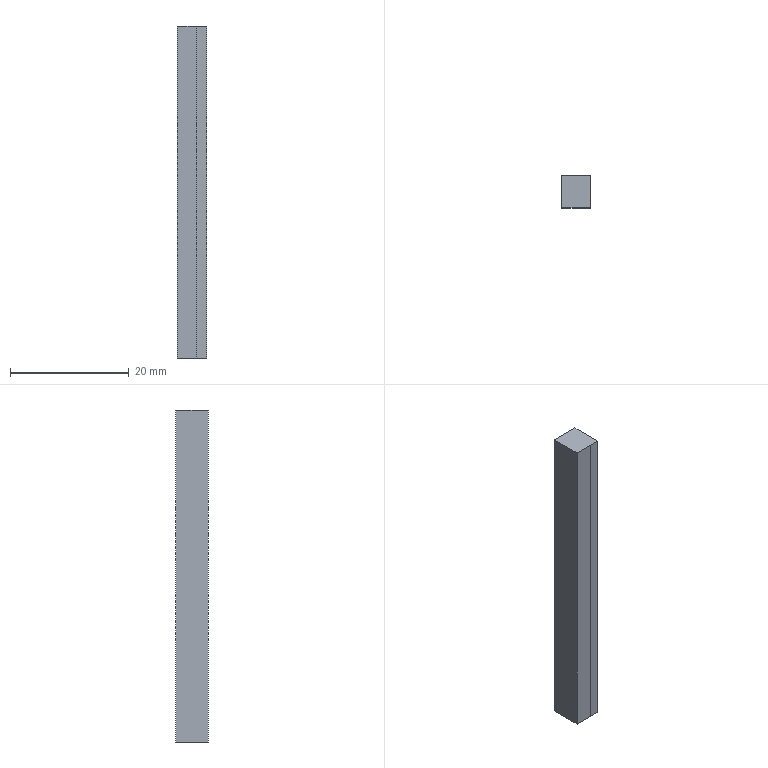Part | NX | features BREP 2 | 2 solids | 14 faces | box 4.903 x 5.406 x 56 mm | volume 2968 mm3 | plane 14
STEP:
#1=CARTESIAN_POINT('',(2.452,2.703,-4.));
#2=VERTEX_POINT('',#1);
#3=CARTESIAN_POINT('',(2.452,2.703,52.));
#4=VERTEX_POINT('',#3);
#5=CARTESIAN_POINT('',(2.452,2.703,0.));
#6=DIRECTION('',(0.,0.,1.));
#7=VECTOR('',#6,1000.);
#8=LINE('',#5,#7);
#9=EDGE_CURVE('',#2,#4,#8,.T.);
#10=ORIENTED_EDGE('',*,*,#9,.T.);
#11=CARTESIAN_POINT('',(2.452,-2.697,52.));
#12=VERTEX_POINT('',#11);
#13=CARTESIAN_POINT('',(2.452,24.305,52.));
#14=DIRECTION('',(0.,1.,0.));
#15=VECTOR('',#14,1000.);
#16=LINE('',#13,#15);
#17=EDGE_CURVE('',#12,#4,#16,.T.);
#18=ORIENTED_EDGE('',*,*,#17,.F.);
#19=CARTESIAN_POINT('',(2.452,-2.697,-4.));
#20=VERTEX_POINT('',#19);
#21=CARTESIAN_POINT('',(2.452,-2.697,0.));
#22=DIRECTION('',(0.,0.,1.));
#23=VECTOR('',#22,1000.);
#24=LINE('',#21,#23);
#25=EDGE_CURVE('',#20,#12,#24,.T.);
#26=ORIENTED_EDGE('',*,*,#25,.F.);
#27=CARTESIAN_POINT('',(2.452,24.305,-4.));
#28=DIRECTION('',(0.,1.,0.));
#29=VECTOR('',#28,1000.);
#30=LINE('',#27,#29);
#31=EDGE_CURVE('',#20,#2,#30,.T.);
#32=ORIENTED_EDGE('',*,*,#31,.T.);
#33=EDGE_LOOP('',(#10,#18,#26,#32));
#34=FACE_BOUND('',#33,.T.);
#35=CARTESIAN_POINT('',(2.452,2.703,0.));
#36=DIRECTION('',(-1.,0.,0.));
#37=DIRECTION('',(0.,1.,0.));
#38=AXIS2_PLACEMENT_3D('',#35,#36,#37);
#39=PLANE('',#38);
#40=ADVANCED_FACE('',(#34),#39,.F.);
#41=CARTESIAN_POINT('',(0.7484,-2.7,-4.));
#42=VERTEX_POINT('',#41);
#43=CARTESIAN_POINT('',(0.7484,-2.7,52.));
#44=VERTEX_POINT('',#43);
#45=CARTESIAN_POINT('',(0.7484,-2.697,52.));
#46=CARTESIAN_POINT('',(0.7484,-2.697,33.333));
#47=CARTESIAN_POINT('',(0.7484,-2.697,14.667));
#48=CARTESIAN_POINT('',(0.7484,-2.697,-4.));
#49=B_SPLINE_CURVE_WITH_KNOTS('',3,(#45,#46,#47,#48),.UNSPECIFIED.,.F.,.F.,(4,4),(0.,1.),.UNSPECIFIED.);
#50=EDGE_CURVE('',#42,#44,#49,.F.);
#51=ORIENTED_EDGE('',*,*,#50,.F.);
#52=CARTESIAN_POINT('',(5.622,-2.697,-4.));
#53=DIRECTION('',(1.,0.,0.));
#54=VECTOR('',#53,1000.);
#55=LINE('',#52,#54);
#56=EDGE_CURVE('',#42,#20,#55,.T.);
#57=ORIENTED_EDGE('',*,*,#56,.T.);
#58=ORIENTED_EDGE('',*,*,#25,.T.);
#59=CARTESIAN_POINT('',(5.622,-2.697,52.));
#60=DIRECTION('',(1.,0.,0.));
#61=VECTOR('',#60,1000.);
#62=LINE('',#59,#61);
#63=EDGE_CURVE('',#44,#12,#62,.T.);
#64=ORIENTED_EDGE('',*,*,#63,.F.);
#65=EDGE_LOOP('',(#51,#57,#58,#64));
#66=FACE_BOUND('',#65,.T.);
#67=CARTESIAN_POINT('',(1.952,-2.697,0.));
#68=DIRECTION('',(0.,1.,0.));
#69=DIRECTION('',(1.,0.,0.));
#70=AXIS2_PLACEMENT_3D('',#67,#68,#69);
#71=PLANE('',#70);
#72=ADVANCED_FACE('',(#66),#71,.F.);
#73=ORIENTED_EDGE('',*,*,#50,.T.);
#74=CARTESIAN_POINT('',(-2.452,-2.703,52.));
#75=VERTEX_POINT('',#74);
#76=CARTESIAN_POINT('',(5.622,-2.703,52.));
#77=DIRECTION('',(1.,0.,0.));
#78=VECTOR('',#77,1000.);
#79=LINE('',#76,#78);
#80=EDGE_CURVE('',#75,#44,#79,.T.);
#81=ORIENTED_EDGE('',*,*,#80,.F.);
#82=CARTESIAN_POINT('',(-2.452,-2.703,-4.));
#83=VERTEX_POINT('',#82);
#84=CARTESIAN_POINT('',(-2.452,-2.703,0.));
#85=DIRECTION('',(0.,0.,1.));
#86=VECTOR('',#85,1000.);
#87=LINE('',#84,#86);
#88=EDGE_CURVE('',#83,#75,#87,.T.);
#89=ORIENTED_EDGE('',*,*,#88,.F.);
#90=CARTESIAN_POINT('',(5.622,-2.703,-4.));
#91=DIRECTION('',(1.,0.,0.));
#92=VECTOR('',#91,1000.);
#93=LINE('',#90,#92);
#94=EDGE_CURVE('',#83,#42,#93,.T.);
#95=ORIENTED_EDGE('',*,*,#94,.T.);
#96=EDGE_LOOP('',(#73,#81,#89,#95));
#97=FACE_BOUND('',#96,.T.);
#98=CARTESIAN_POINT('',(0.7484,-2.703,0.));
#99=DIRECTION('',(0.,1.,0.));
#100=DIRECTION('',(1.,0.,0.));
#101=AXIS2_PLACEMENT_3D('',#98,#99,#100);
#102=PLANE('',#101);
#103=ADVANCED_FACE('',(#97),#102,.F.);
#104=ORIENTED_EDGE('',*,*,#88,.T.);
#105=CARTESIAN_POINT('',(-2.452,2.703,52.));
#106=VERTEX_POINT('',#105);
#107=CARTESIAN_POINT('',(-2.452,24.305,52.));
#108=DIRECTION('',(0.,-1.,0.));
#109=VECTOR('',#108,1000.);
#110=LINE('',#107,#109);
#111=EDGE_CURVE('',#106,#75,#110,.T.);
#112=ORIENTED_EDGE('',*,*,#111,.F.);
#113=CARTESIAN_POINT('',(-2.452,2.703,-4.));
#114=VERTEX_POINT('',#113);
#115=CARTESIAN_POINT('',(-2.452,2.703,0.));
#116=DIRECTION('',(0.,0.,1.));
#117=VECTOR('',#116,1000.);
#118=LINE('',#115,#117);
#119=EDGE_CURVE('',#114,#106,#118,.T.);
#120=ORIENTED_EDGE('',*,*,#119,.F.);
#121=CARTESIAN_POINT('',(-2.452,24.305,-4.));
#122=DIRECTION('',(0.,-1.,0.));
#123=VECTOR('',#122,1000.);
#124=LINE('',#121,#123);
#125=EDGE_CURVE('',#114,#83,#124,.T.);
#126=ORIENTED_EDGE('',*,*,#125,.T.);
#127=EDGE_LOOP('',(#104,#112,#120,#126));
#128=FACE_BOUND('',#127,.T.);
#129=CARTESIAN_POINT('',(-2.452,-2.703,0.));
#130=DIRECTION('',(1.,0.,0.));
#131=DIRECTION('',(0.,-1.,0.));
#132=AXIS2_PLACEMENT_3D('',#129,#130,#131);
#133=PLANE('',#132);
#134=ADVANCED_FACE('',(#128),#133,.F.);
#135=CARTESIAN_POINT('',(5.622,2.703,-4.));
#136=DIRECTION('',(-1.,0.,0.));
#137=VECTOR('',#136,1000.);
#138=LINE('',#135,#137);
#139=EDGE_CURVE('',#2,#114,#138,.T.);
#140=ORIENTED_EDGE('',*,*,#139,.T.);
#141=ORIENTED_EDGE('',*,*,#119,.T.);
#142=CARTESIAN_POINT('',(5.622,2.703,52.));
#143=DIRECTION('',(-1.,0.,0.));
#144=VECTOR('',#143,1000.);
#145=LINE('',#142,#144);
#146=EDGE_CURVE('',#4,#106,#145,.T.);
#147=ORIENTED_EDGE('',*,*,#146,.F.);
#148=ORIENTED_EDGE('',*,*,#9,.F.);
#149=EDGE_LOOP('',(#140,#141,#147,#148));
#150=FACE_BOUND('',#149,.T.);
#151=CARTESIAN_POINT('',(0.7484,2.703,0.));
#152=DIRECTION('',(0.,-1.,0.));
#153=DIRECTION('',(-1.,0.,0.));
#154=AXIS2_PLACEMENT_3D('',#151,#152,#153);
#155=PLANE('',#154);
#156=ADVANCED_FACE('',(#150),#155,.F.);
#157=ORIENTED_EDGE('',*,*,#146,.T.);
#158=ORIENTED_EDGE('',*,*,#111,.T.);
#159=ORIENTED_EDGE('',*,*,#80,.T.);
#160=ORIENTED_EDGE('',*,*,#63,.T.);
#161=ORIENTED_EDGE('',*,*,#17,.T.);
#162=EDGE_LOOP('',(#157,#158,#159,#160,#161));
#163=FACE_BOUND('',#162,.T.);
#164=CARTESIAN_POINT('',(5.622,24.305,52.));
#165=DIRECTION('',(0.,0.,1.));
#166=DIRECTION('',(-1.,0.,0.));
#167=AXIS2_PLACEMENT_3D('',#164,#165,#166);
#168=PLANE('',#167);
#169=ADVANCED_FACE('',(#163),#168,.T.);
#170=ORIENTED_EDGE('',*,*,#125,.F.);
#171=ORIENTED_EDGE('',*,*,#139,.F.);
#172=ORIENTED_EDGE('',*,*,#31,.F.);
#173=ORIENTED_EDGE('',*,*,#56,.F.);
#174=ORIENTED_EDGE('',*,*,#94,.F.);
#175=EDGE_LOOP('',(#170,#171,#172,#173,#174));
#176=FACE_BOUND('',#175,.T.);
#177=CARTESIAN_POINT('',(5.622,24.305,-4.));
#178=DIRECTION('',(0.,0.,1.));
#179=DIRECTION('',(-1.,0.,0.));
#180=AXIS2_PLACEMENT_3D('',#177,#178,#179);
#181=PLANE('',#180);
#182=ADVANCED_FACE('',(#176),#181,.F.);
#183=CLOSED_SHELL('',(#40,#72,#103,#134,#156,#169,#182));
#184=MANIFOLD_SOLID_BREP('',#183);
#185=CARTESIAN_POINT('',(2.452,2.703,-4.));
#186=VERTEX_POINT('',#185);
#187=CARTESIAN_POINT('',(2.452,2.703,52.));
#188=VERTEX_POINT('',#187);
#189=CARTESIAN_POINT('',(2.452,2.703,0.));
#190=DIRECTION('',(0.,0.,1.));
#191=VECTOR('',#190,1000.);
#192=LINE('',#189,#191);
#193=EDGE_CURVE('',#186,#188,#192,.T.);
#194=ORIENTED_EDGE('',*,*,#193,.T.);
#195=CARTESIAN_POINT('',(2.452,-2.697,52.));
#196=VERTEX_POINT('',#195);
#197=CARTESIAN_POINT('',(2.452,24.305,52.));
#198=DIRECTION('',(0.,1.,0.));
#199=VECTOR('',#198,1000.);
#200=LINE('',#197,#199);
#201=EDGE_CURVE('',#196,#188,#200,.T.);
#202=ORIENTED_EDGE('',*,*,#201,.F.);
#203=CARTESIAN_POINT('',(2.452,-2.697,-4.));
#204=VERTEX_POINT('',#203);
#205=CARTESIAN_POINT('',(2.452,-2.697,0.));
#206=DIRECTION('',(0.,0.,1.));
#207=VECTOR('',#206,1000.);
#208=LINE('',#205,#207);
#209=EDGE_CURVE('',#204,#196,#208,.T.);
#210=ORIENTED_EDGE('',*,*,#209,.F.);
#211=CARTESIAN_POINT('',(2.452,24.305,-4.));
#212=DIRECTION('',(0.,1.,0.));
#213=VECTOR('',#212,1000.);
#214=LINE('',#211,#213);
#215=EDGE_CURVE('',#204,#186,#214,.T.);
#216=ORIENTED_EDGE('',*,*,#215,.T.);
#217=EDGE_LOOP('',(#194,#202,#210,#216));
#218=FACE_BOUND('',#217,.T.);
#219=CARTESIAN_POINT('',(2.452,2.703,0.));
#220=DIRECTION('',(-1.,0.,0.));
#221=DIRECTION('',(0.,1.,0.));
#222=AXIS2_PLACEMENT_3D('',#219,#220,#221);
#223=PLANE('',#222);
#224=ADVANCED_FACE('',(#218),#223,.F.);
#225=CARTESIAN_POINT('',(0.7484,-2.7,-4.));
#226=VERTEX_POINT('',#225);
#227=CARTESIAN_POINT('',(0.7484,-2.7,52.));
#228=VERTEX_POINT('',#227);
#229=CARTESIAN_POINT('',(0.7484,-2.697,52.));
#230=CARTESIAN_POINT('',(0.7484,-2.697,33.333));
#231=CARTESIAN_POINT('',(0.7484,-2.697,14.667));
#232=CARTESIAN_POINT('',(0.7484,-2.697,-4.));
#233=B_SPLINE_CURVE_WITH_KNOTS('',3,(#229,#230,#231,#232),.UNSPECIFIED.,.F.,.F.,(4,4),(0.,1.),.UNSPECIFIED.);
#234=EDGE_CURVE('',#226,#228,#233,.F.);
#235=ORIENTED_EDGE('',*,*,#234,.F.);
#236=CARTESIAN_POINT('',(5.622,-2.697,-4.));
#237=DIRECTION('',(1.,0.,0.));
#238=VECTOR('',#237,1000.);
#239=LINE('',#236,#238);
#240=EDGE_CURVE('',#226,#204,#239,.T.);
#241=ORIENTED_EDGE('',*,*,#240,.T.);
#242=ORIENTED_EDGE('',*,*,#209,.T.);
#243=CARTESIAN_POINT('',(5.622,-2.697,52.));
#244=DIRECTION('',(1.,0.,0.));
#245=VECTOR('',#244,1000.);
#246=LINE('',#243,#245);
#247=EDGE_CURVE('',#228,#196,#246,.T.);
#248=ORIENTED_EDGE('',*,*,#247,.F.);
#249=EDGE_LOOP('',(#235,#241,#242,#248));
#250=FACE_BOUND('',#249,.T.);
#251=CARTESIAN_POINT('',(1.952,-2.697,0.));
#252=DIRECTION('',(0.,1.,0.));
#253=DIRECTION('',(1.,0.,0.));
#254=AXIS2_PLACEMENT_3D('',#251,#252,#253);
#255=PLANE('',#254);
#256=ADVANCED_FACE('',(#250),#255,.F.);
#257=ORIENTED_EDGE('',*,*,#234,.T.);
#258=CARTESIAN_POINT('',(-2.452,-2.703,52.));
#259=VERTEX_POINT('',#258);
#260=CARTESIAN_POINT('',(5.622,-2.703,52.));
#261=DIRECTION('',(1.,0.,0.));
#262=VECTOR('',#261,1000.);
#263=LINE('',#260,#262);
#264=EDGE_CURVE('',#259,#228,#263,.T.);
#265=ORIENTED_EDGE('',*,*,#264,.F.);
#266=CARTESIAN_POINT('',(-2.452,-2.703,-4.));
#267=VERTEX_POINT('',#266);
#268=CARTESIAN_POINT('',(-2.452,-2.703,0.));
#269=DIRECTION('',(0.,0.,1.));
#270=VECTOR('',#269,1000.);
#271=LINE('',#268,#270);
#272=EDGE_CURVE('',#267,#259,#271,.T.);
#273=ORIENTED_EDGE('',*,*,#272,.F.);
#274=CARTESIAN_POINT('',(5.622,-2.703,-4.));
#275=DIRECTION('',(1.,0.,0.));
#276=VECTOR('',#275,1000.);
#277=LINE('',#274,#276);
#278=EDGE_CURVE('',#267,#226,#277,.T.);
#279=ORIENTED_EDGE('',*,*,#278,.T.);
#280=EDGE_LOOP('',(#257,#265,#273,#279));
#281=FACE_BOUND('',#280,.T.);
#282=CARTESIAN_POINT('',(0.7484,-2.703,0.));
#283=DIRECTION('',(0.,1.,0.));
#284=DIRECTION('',(1.,0.,0.));
#285=AXIS2_PLACEMENT_3D('',#282,#283,#284);
#286=PLANE('',#285);
#287=ADVANCED_FACE('',(#281),#286,.F.);
#288=ORIENTED_EDGE('',*,*,#272,.T.);
#289=CARTESIAN_POINT('',(-2.452,2.703,52.));
#290=VERTEX_POINT('',#289);
#291=CARTESIAN_POINT('',(-2.452,24.305,52.));
#292=DIRECTION('',(0.,-1.,0.));
#293=VECTOR('',#292,1000.);
#294=LINE('',#291,#293);
#295=EDGE_CURVE('',#290,#259,#294,.T.);
#296=ORIENTED_EDGE('',*,*,#295,.F.);
#297=CARTESIAN_POINT('',(-2.452,2.703,-4.));
#298=VERTEX_POINT('',#297);
#299=CARTESIAN_POINT('',(-2.452,2.703,0.));
#300=DIRECTION('',(0.,0.,1.));
#301=VECTOR('',#300,1000.);
#302=LINE('',#299,#301);
#303=EDGE_CURVE('',#298,#290,#302,.T.);
#304=ORIENTED_EDGE('',*,*,#303,.F.);
#305=CARTESIAN_POINT('',(-2.452,24.305,-4.));
#306=DIRECTION('',(0.,-1.,0.));
#307=VECTOR('',#306,1000.);
#308=LINE('',#305,#307);
#309=EDGE_CURVE('',#298,#267,#308,.T.);
#310=ORIENTED_EDGE('',*,*,#309,.T.);
#311=EDGE_LOOP('',(#288,#296,#304,#310));
#312=FACE_BOUND('',#311,.T.);
#313=CARTESIAN_POINT('',(-2.452,-2.703,0.));
#314=DIRECTION('',(1.,0.,0.));
#315=DIRECTION('',(0.,-1.,0.));
#316=AXIS2_PLACEMENT_3D('',#313,#314,#315);
#317=PLANE('',#316);
#318=ADVANCED_FACE('',(#312),#317,.F.);
#319=CARTESIAN_POINT('',(5.622,2.703,-4.));
#320=DIRECTION('',(-1.,0.,0.));
#321=VECTOR('',#320,1000.);
#322=LINE('',#319,#321);
#323=EDGE_CURVE('',#186,#298,#322,.T.);
#324=ORIENTED_EDGE('',*,*,#323,.T.);
#325=ORIENTED_EDGE('',*,*,#303,.T.);
#326=CARTESIAN_POINT('',(5.622,2.703,52.));
#327=DIRECTION('',(-1.,0.,0.));
#328=VECTOR('',#327,1000.);
#329=LINE('',#326,#328);
#330=EDGE_CURVE('',#188,#290,#329,.T.);
#331=ORIENTED_EDGE('',*,*,#330,.F.);
#332=ORIENTED_EDGE('',*,*,#193,.F.);
#333=EDGE_LOOP('',(#324,#325,#331,#332));
#334=FACE_BOUND('',#333,.T.);
#335=CARTESIAN_POINT('',(0.7484,2.703,0.));
#336=DIRECTION('',(0.,-1.,0.));
#337=DIRECTION('',(-1.,0.,0.));
#338=AXIS2_PLACEMENT_3D('',#335,#336,#337);
#339=PLANE('',#338);
#340=ADVANCED_FACE('',(#334),#339,.F.);
#341=ORIENTED_EDGE('',*,*,#330,.T.);
#342=ORIENTED_EDGE('',*,*,#295,.T.);
#343=ORIENTED_EDGE('',*,*,#264,.T.);
#344=ORIENTED_EDGE('',*,*,#247,.T.);
#345=ORIENTED_EDGE('',*,*,#201,.T.);
#346=EDGE_LOOP('',(#341,#342,#343,#344,#345));
#347=FACE_BOUND('',#346,.T.);
#348=CARTESIAN_POINT('',(5.622,24.305,52.));
#349=DIRECTION('',(0.,0.,1.));
#350=DIRECTION('',(-1.,0.,0.));
#351=AXIS2_PLACEMENT_3D('',#348,#349,#350);
#352=PLANE('',#351);
#353=ADVANCED_FACE('',(#347),#352,.T.);
#354=ORIENTED_EDGE('',*,*,#309,.F.);
#355=ORIENTED_EDGE('',*,*,#323,.F.);
#356=ORIENTED_EDGE('',*,*,#215,.F.);
#357=ORIENTED_EDGE('',*,*,#240,.F.);
#358=ORIENTED_EDGE('',*,*,#278,.F.);
#359=EDGE_LOOP('',(#354,#355,#356,#357,#358));
#360=FACE_BOUND('',#359,.T.);
#361=CARTESIAN_POINT('',(5.622,24.305,-4.));
#362=DIRECTION('',(0.,0.,1.));
#363=DIRECTION('',(-1.,0.,0.));
#364=AXIS2_PLACEMENT_3D('',#361,#362,#363);
#365=PLANE('',#364);
#366=ADVANCED_FACE('',(#360),#365,.F.);
#367=CLOSED_SHELL('',(#224,#256,#287,#318,#340,#353,#366));
#368=MANIFOLD_SOLID_BREP('',#367);
#369=(LENGTH_UNIT()NAMED_UNIT(*)SI_UNIT(.MILLI.,.METRE.));
#370=UNCERTAINTY_MEASURE_WITH_UNIT(LENGTH_MEASURE(0.0508),#369,'','');
#371=(NAMED_UNIT(*)PLANE_ANGLE_UNIT()SI_UNIT($,.RADIAN.));
#372=(NAMED_UNIT(*)SI_UNIT($,.STERADIAN.)SOLID_ANGLE_UNIT());
#373=(GEOMETRIC_REPRESENTATION_CONTEXT(3)GLOBAL_UNCERTAINTY_ASSIGNED_CONTEXT((#370))GLOBAL_UNIT_ASSIGNED_CONTEXT((#369,#371,#372))REPRESENTATION_CONTEXT('',''));
#374=ADVANCED_BREP_SHAPE_REPRESENTATION('',(#184,#368),#373);